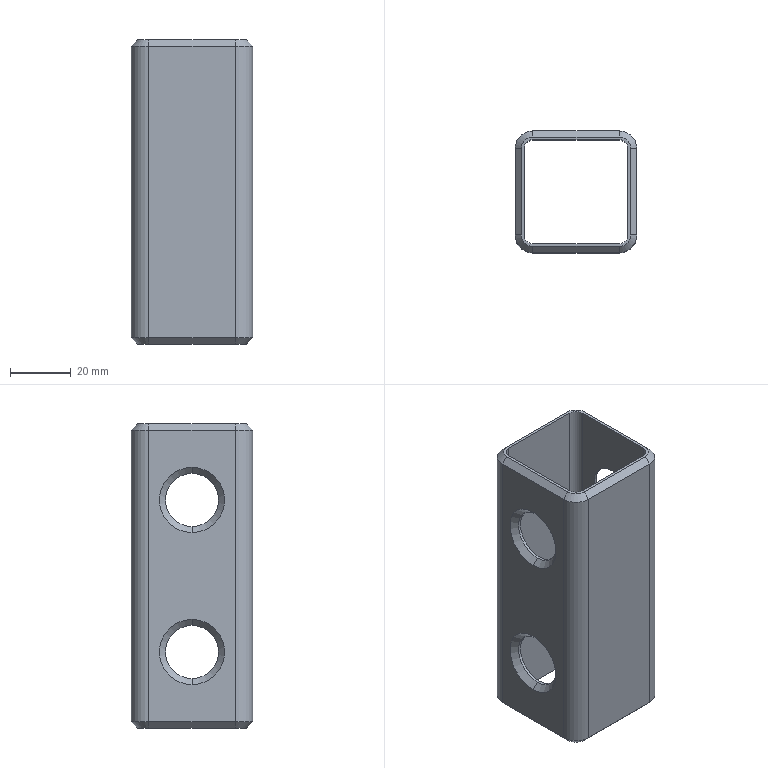Part | STEP file | IN-01-01-04-05 | 1 solid | 50 faces | box 40 x 40 x 100 mm | volume 37023 mm3 | plane 18 | cylinder 16 | cone 16 | commonest cylinder face diameters 17.5 x8 5.8 x4 11.6 x4